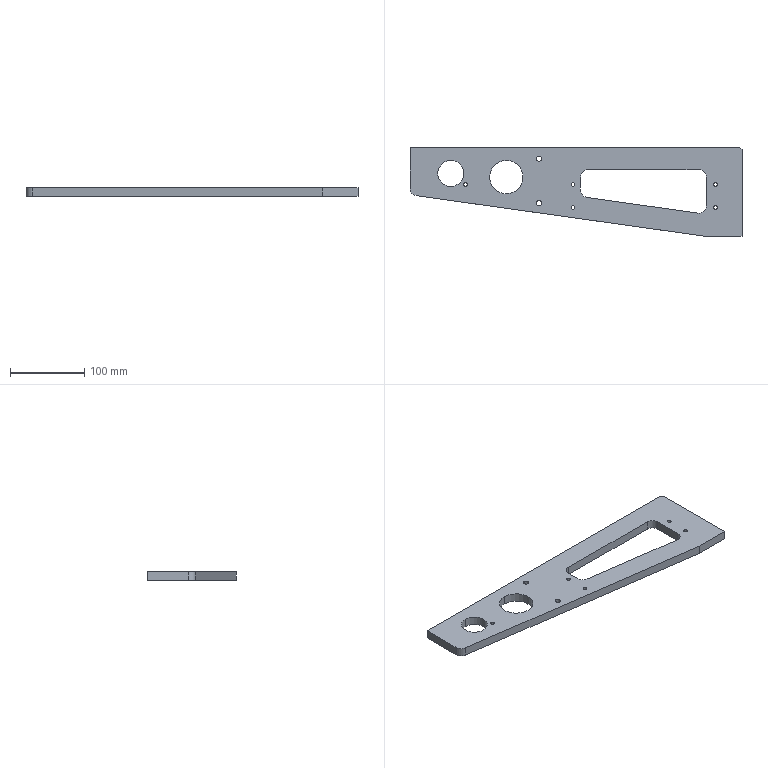Part | STEP file | J454-EBZ05-32-03 | 1 solid | 91 faces | box 448 x 120 x 12 mm | volume 376287 mm3 | cylinder 55 | plane 20 | cone 16 | commonest cylinder face diameters 5.1 x16 6 x16 5 x10 20 x5 7 x4 35 x2